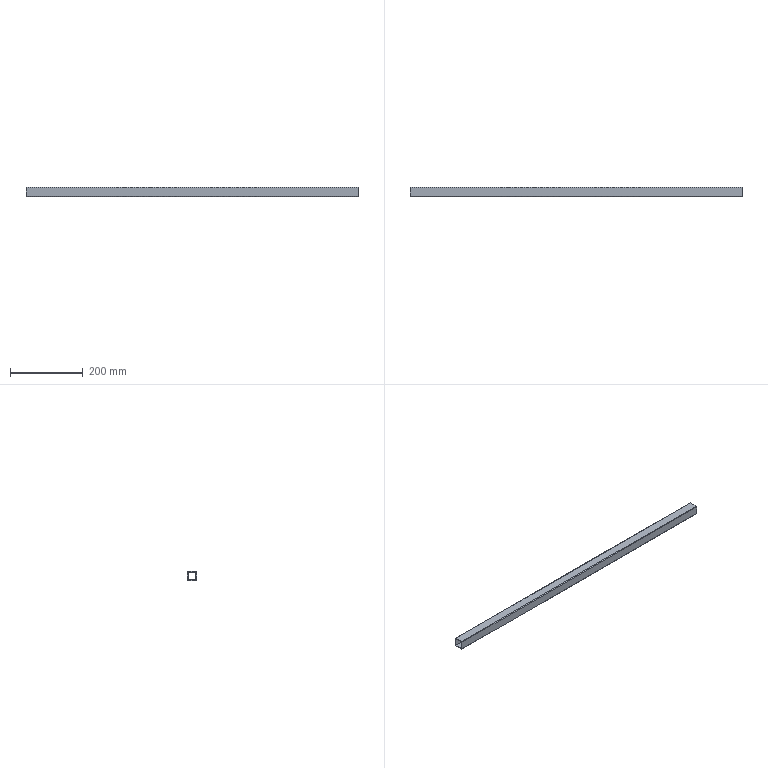Part | NX | features BREP 1 | 1 solid | 14 faces | box 910.59 x 25.4 x 25.4 mm | volume 159055 mm3 | plane 10 | cylinder 4 | commonest cylinder face diameters 3.175 x4
STEP:
#1=CARTESIAN_POINT('',(-455.295,12.7,-11.113));
#2=VERTEX_POINT('',#1);
#3=CARTESIAN_POINT('',(-455.295,12.7,11.113));
#4=VERTEX_POINT('',#3);
#5=CARTESIAN_POINT('',(-455.295,12.7,-11.113));
#6=DIRECTION('',(0.,0.,1.));
#7=VECTOR('',#6,1000.);
#8=LINE('',#5,#7);
#9=EDGE_CURVE('',#2,#4,#8,.T.);
#10=ORIENTED_EDGE('',*,*,#9,.F.);
#11=CARTESIAN_POINT('',(-455.295,11.113,-12.7));
#12=VERTEX_POINT('',#11);
#13=CARTESIAN_POINT('',(-455.295,11.113,-11.113));
#14=DIRECTION('',(-1.,0.,0.));
#15=DIRECTION('',(0.,1.,0.));
#16=AXIS2_PLACEMENT_3D('',#13,#14,#15);
#17=CIRCLE('',#16,1.587);
#18=EDGE_CURVE('',#2,#12,#17,.T.);
#19=ORIENTED_EDGE('',*,*,#18,.T.);
#20=CARTESIAN_POINT('',(-455.295,-11.113,-12.7));
#21=VERTEX_POINT('',#20);
#22=CARTESIAN_POINT('',(-455.295,-11.113,-12.7));
#23=DIRECTION('',(0.,1.,0.));
#24=VECTOR('',#23,1000.);
#25=LINE('',#22,#24);
#26=EDGE_CURVE('',#21,#12,#25,.T.);
#27=ORIENTED_EDGE('',*,*,#26,.F.);
#28=CARTESIAN_POINT('',(-455.295,-12.7,-11.113));
#29=VERTEX_POINT('',#28);
#30=CARTESIAN_POINT('',(-455.295,-11.113,-11.113));
#31=DIRECTION('',(-1.,0.,0.));
#32=DIRECTION('',(0.,0.,-1.));
#33=AXIS2_PLACEMENT_3D('',#30,#31,#32);
#34=CIRCLE('',#33,1.587);
#35=EDGE_CURVE('',#21,#29,#34,.T.);
#36=ORIENTED_EDGE('',*,*,#35,.T.);
#37=CARTESIAN_POINT('',(-455.295,-12.7,11.113));
#38=VERTEX_POINT('',#37);
#39=CARTESIAN_POINT('',(-455.295,-12.7,11.113));
#40=DIRECTION('',(0.,0.,-1.));
#41=VECTOR('',#40,1000.);
#42=LINE('',#39,#41);
#43=EDGE_CURVE('',#38,#29,#42,.T.);
#44=ORIENTED_EDGE('',*,*,#43,.F.);
#45=CARTESIAN_POINT('',(-455.295,-11.113,12.7));
#46=VERTEX_POINT('',#45);
#47=CARTESIAN_POINT('',(-455.295,-11.113,11.113));
#48=DIRECTION('',(-1.,0.,0.));
#49=DIRECTION('',(0.,-1.,0.));
#50=AXIS2_PLACEMENT_3D('',#47,#48,#49);
#51=CIRCLE('',#50,1.587);
#52=EDGE_CURVE('',#38,#46,#51,.T.);
#53=ORIENTED_EDGE('',*,*,#52,.T.);
#54=CARTESIAN_POINT('',(-455.295,11.113,12.7));
#55=VERTEX_POINT('',#54);
#56=CARTESIAN_POINT('',(-455.295,11.113,12.7));
#57=DIRECTION('',(0.,-1.,0.));
#58=VECTOR('',#57,1000.);
#59=LINE('',#56,#58);
#60=EDGE_CURVE('',#55,#46,#59,.T.);
#61=ORIENTED_EDGE('',*,*,#60,.F.);
#62=CARTESIAN_POINT('',(-455.295,11.113,11.113));
#63=DIRECTION('',(-1.,0.,0.));
#64=DIRECTION('',(0.,0.,1.));
#65=AXIS2_PLACEMENT_3D('',#62,#63,#64);
#66=CIRCLE('',#65,1.587);
#67=EDGE_CURVE('',#55,#4,#66,.T.);
#68=ORIENTED_EDGE('',*,*,#67,.T.);
#69=EDGE_LOOP('',(#10,#19,#27,#36,#44,#53,#61,#68));
#70=FACE_BOUND('',#69,.T.);
#71=CARTESIAN_POINT('',(-455.295,10.82,10.82));
#72=VERTEX_POINT('',#71);
#73=CARTESIAN_POINT('',(-455.295,10.82,-10.82));
#74=VERTEX_POINT('',#73);
#75=CARTESIAN_POINT('',(-455.295,10.82,10.82));
#76=DIRECTION('',(0.,0.,-1.));
#77=VECTOR('',#76,1000.);
#78=LINE('',#75,#77);
#79=EDGE_CURVE('',#72,#74,#78,.T.);
#80=ORIENTED_EDGE('',*,*,#79,.F.);
#81=CARTESIAN_POINT('',(-455.295,-10.82,10.82));
#82=VERTEX_POINT('',#81);
#83=CARTESIAN_POINT('',(-455.295,-10.82,10.82));
#84=DIRECTION('',(0.,1.,0.));
#85=VECTOR('',#84,1000.);
#86=LINE('',#83,#85);
#87=EDGE_CURVE('',#82,#72,#86,.T.);
#88=ORIENTED_EDGE('',*,*,#87,.F.);
#89=CARTESIAN_POINT('',(-455.295,-10.82,-10.82));
#90=VERTEX_POINT('',#89);
#91=CARTESIAN_POINT('',(-455.295,-10.82,-10.82));
#92=DIRECTION('',(0.,0.,1.));
#93=VECTOR('',#92,1000.);
#94=LINE('',#91,#93);
#95=EDGE_CURVE('',#90,#82,#94,.T.);
#96=ORIENTED_EDGE('',*,*,#95,.F.);
#97=CARTESIAN_POINT('',(-455.295,10.82,-10.82));
#98=DIRECTION('',(0.,-1.,0.));
#99=VECTOR('',#98,1000.);
#100=LINE('',#97,#99);
#101=EDGE_CURVE('',#74,#90,#100,.T.);
#102=ORIENTED_EDGE('',*,*,#101,.F.);
#103=EDGE_LOOP('',(#80,#88,#96,#102));
#104=FACE_BOUND('',#103,.T.);
#105=CARTESIAN_POINT('',(-455.295,0.,0.));
#106=DIRECTION('',(1.,0.,0.));
#107=DIRECTION('',(0.,1.,0.));
#108=AXIS2_PLACEMENT_3D('',#105,#106,#107);
#109=PLANE('',#108);
#110=ADVANCED_FACE('',(#70,#104),#109,.F.);
#111=CARTESIAN_POINT('',(455.295,-10.82,-10.82));
#112=VERTEX_POINT('',#111);
#113=CARTESIAN_POINT('',(-455.295,-10.82,-10.82));
#114=DIRECTION('',(1.,0.,0.));
#115=VECTOR('',#114,1000.);
#116=LINE('',#113,#115);
#117=EDGE_CURVE('',#90,#112,#116,.T.);
#118=ORIENTED_EDGE('',*,*,#117,.T.);
#119=CARTESIAN_POINT('',(455.295,10.82,-10.82));
#120=VERTEX_POINT('',#119);
#121=CARTESIAN_POINT('',(455.295,10.82,-10.82));
#122=DIRECTION('',(0.,-1.,0.));
#123=VECTOR('',#122,1000.);
#124=LINE('',#121,#123);
#125=EDGE_CURVE('',#120,#112,#124,.T.);
#126=ORIENTED_EDGE('',*,*,#125,.F.);
#127=CARTESIAN_POINT('',(-455.295,10.82,-10.82));
#128=DIRECTION('',(1.,0.,0.));
#129=VECTOR('',#128,1000.);
#130=LINE('',#127,#129);
#131=EDGE_CURVE('',#74,#120,#130,.T.);
#132=ORIENTED_EDGE('',*,*,#131,.F.);
#133=ORIENTED_EDGE('',*,*,#101,.T.);
#134=EDGE_LOOP('',(#118,#126,#132,#133));
#135=FACE_BOUND('',#134,.T.);
#136=CARTESIAN_POINT('',(-455.295,10.82,-10.82));
#137=DIRECTION('',(0.,0.,1.));
#138=DIRECTION('',(1.,0.,0.));
#139=AXIS2_PLACEMENT_3D('',#136,#137,#138);
#140=PLANE('',#139);
#141=ADVANCED_FACE('',(#135),#140,.T.);
#142=ORIENTED_EDGE('',*,*,#131,.T.);
#143=CARTESIAN_POINT('',(455.295,10.82,10.82));
#144=VERTEX_POINT('',#143);
#145=CARTESIAN_POINT('',(455.295,10.82,10.82));
#146=DIRECTION('',(0.,0.,-1.));
#147=VECTOR('',#146,1000.);
#148=LINE('',#145,#147);
#149=EDGE_CURVE('',#144,#120,#148,.T.);
#150=ORIENTED_EDGE('',*,*,#149,.F.);
#151=CARTESIAN_POINT('',(-455.295,10.82,10.82));
#152=DIRECTION('',(1.,0.,0.));
#153=VECTOR('',#152,1000.);
#154=LINE('',#151,#153);
#155=EDGE_CURVE('',#72,#144,#154,.T.);
#156=ORIENTED_EDGE('',*,*,#155,.F.);
#157=ORIENTED_EDGE('',*,*,#79,.T.);
#158=EDGE_LOOP('',(#142,#150,#156,#157));
#159=FACE_BOUND('',#158,.T.);
#160=CARTESIAN_POINT('',(-455.295,10.82,10.82));
#161=DIRECTION('',(0.,-1.,0.));
#162=DIRECTION('',(0.,0.,-1.));
#163=AXIS2_PLACEMENT_3D('',#160,#161,#162);
#164=PLANE('',#163);
#165=ADVANCED_FACE('',(#159),#164,.T.);
#166=ORIENTED_EDGE('',*,*,#155,.T.);
#167=CARTESIAN_POINT('',(455.295,-10.82,10.82));
#168=VERTEX_POINT('',#167);
#169=CARTESIAN_POINT('',(455.295,-10.82,10.82));
#170=DIRECTION('',(0.,1.,0.));
#171=VECTOR('',#170,1000.);
#172=LINE('',#169,#171);
#173=EDGE_CURVE('',#168,#144,#172,.T.);
#174=ORIENTED_EDGE('',*,*,#173,.F.);
#175=CARTESIAN_POINT('',(-455.295,-10.82,10.82));
#176=DIRECTION('',(1.,0.,0.));
#177=VECTOR('',#176,1000.);
#178=LINE('',#175,#177);
#179=EDGE_CURVE('',#82,#168,#178,.T.);
#180=ORIENTED_EDGE('',*,*,#179,.F.);
#181=ORIENTED_EDGE('',*,*,#87,.T.);
#182=EDGE_LOOP('',(#166,#174,#180,#181));
#183=FACE_BOUND('',#182,.T.);
#184=CARTESIAN_POINT('',(-455.295,-10.82,10.82));
#185=DIRECTION('',(0.,0.,-1.));
#186=DIRECTION('',(0.,-1.,0.));
#187=AXIS2_PLACEMENT_3D('',#184,#185,#186);
#188=PLANE('',#187);
#189=ADVANCED_FACE('',(#183),#188,.T.);
#190=ORIENTED_EDGE('',*,*,#179,.T.);
#191=CARTESIAN_POINT('',(455.295,-10.82,-10.82));
#192=DIRECTION('',(0.,0.,1.));
#193=VECTOR('',#192,1000.);
#194=LINE('',#191,#193);
#195=EDGE_CURVE('',#112,#168,#194,.T.);
#196=ORIENTED_EDGE('',*,*,#195,.F.);
#197=ORIENTED_EDGE('',*,*,#117,.F.);
#198=ORIENTED_EDGE('',*,*,#95,.T.);
#199=EDGE_LOOP('',(#190,#196,#197,#198));
#200=FACE_BOUND('',#199,.T.);
#201=CARTESIAN_POINT('',(-455.295,-10.82,-10.82));
#202=DIRECTION('',(0.,1.,0.));
#203=DIRECTION('',(1.,0.,0.));
#204=AXIS2_PLACEMENT_3D('',#201,#202,#203);
#205=PLANE('',#204);
#206=ADVANCED_FACE('',(#200),#205,.T.);
#207=CARTESIAN_POINT('',(455.295,11.113,12.7));
#208=VERTEX_POINT('',#207);
#209=CARTESIAN_POINT('',(455.295,-11.113,12.7));
#210=VERTEX_POINT('',#209);
#211=CARTESIAN_POINT('',(455.295,11.113,12.7));
#212=DIRECTION('',(0.,-1.,0.));
#213=VECTOR('',#212,1000.);
#214=LINE('',#211,#213);
#215=EDGE_CURVE('',#208,#210,#214,.T.);
#216=ORIENTED_EDGE('',*,*,#215,.T.);
#217=CARTESIAN_POINT('',(455.295,-12.7,11.113));
#218=VERTEX_POINT('',#217);
#219=CARTESIAN_POINT('',(455.295,-11.113,11.113));
#220=DIRECTION('',(1.,0.,0.));
#221=DIRECTION('',(0.,0.,1.));
#222=AXIS2_PLACEMENT_3D('',#219,#220,#221);
#223=CIRCLE('',#222,1.587);
#224=EDGE_CURVE('',#210,#218,#223,.T.);
#225=ORIENTED_EDGE('',*,*,#224,.T.);
#226=CARTESIAN_POINT('',(455.295,-12.7,-11.113));
#227=VERTEX_POINT('',#226);
#228=CARTESIAN_POINT('',(455.295,-12.7,11.113));
#229=DIRECTION('',(0.,0.,-1.));
#230=VECTOR('',#229,1000.);
#231=LINE('',#228,#230);
#232=EDGE_CURVE('',#218,#227,#231,.T.);
#233=ORIENTED_EDGE('',*,*,#232,.T.);
#234=CARTESIAN_POINT('',(455.295,-11.113,-12.7));
#235=VERTEX_POINT('',#234);
#236=CARTESIAN_POINT('',(455.295,-11.113,-11.113));
#237=DIRECTION('',(1.,0.,0.));
#238=DIRECTION('',(0.,-1.,0.));
#239=AXIS2_PLACEMENT_3D('',#236,#237,#238);
#240=CIRCLE('',#239,1.587);
#241=EDGE_CURVE('',#227,#235,#240,.T.);
#242=ORIENTED_EDGE('',*,*,#241,.T.);
#243=CARTESIAN_POINT('',(455.295,11.113,-12.7));
#244=VERTEX_POINT('',#243);
#245=CARTESIAN_POINT('',(455.295,-11.113,-12.7));
#246=DIRECTION('',(0.,1.,0.));
#247=VECTOR('',#246,1000.);
#248=LINE('',#245,#247);
#249=EDGE_CURVE('',#235,#244,#248,.T.);
#250=ORIENTED_EDGE('',*,*,#249,.T.);
#251=CARTESIAN_POINT('',(455.295,12.7,-11.113));
#252=VERTEX_POINT('',#251);
#253=CARTESIAN_POINT('',(455.295,11.113,-11.113));
#254=DIRECTION('',(1.,0.,0.));
#255=DIRECTION('',(0.,0.,-1.));
#256=AXIS2_PLACEMENT_3D('',#253,#254,#255);
#257=CIRCLE('',#256,1.587);
#258=EDGE_CURVE('',#244,#252,#257,.T.);
#259=ORIENTED_EDGE('',*,*,#258,.T.);
#260=CARTESIAN_POINT('',(455.295,12.7,11.113));
#261=VERTEX_POINT('',#260);
#262=CARTESIAN_POINT('',(455.295,12.7,-11.113));
#263=DIRECTION('',(0.,0.,1.));
#264=VECTOR('',#263,1000.);
#265=LINE('',#262,#264);
#266=EDGE_CURVE('',#252,#261,#265,.T.);
#267=ORIENTED_EDGE('',*,*,#266,.T.);
#268=CARTESIAN_POINT('',(455.295,11.113,11.113));
#269=DIRECTION('',(1.,0.,0.));
#270=DIRECTION('',(0.,1.,0.));
#271=AXIS2_PLACEMENT_3D('',#268,#269,#270);
#272=CIRCLE('',#271,1.587);
#273=EDGE_CURVE('',#261,#208,#272,.T.);
#274=ORIENTED_EDGE('',*,*,#273,.T.);
#275=EDGE_LOOP('',(#216,#225,#233,#242,#250,#259,#267,#274));
#276=FACE_BOUND('',#275,.T.);
#277=ORIENTED_EDGE('',*,*,#195,.T.);
#278=ORIENTED_EDGE('',*,*,#173,.T.);
#279=ORIENTED_EDGE('',*,*,#149,.T.);
#280=ORIENTED_EDGE('',*,*,#125,.T.);
#281=EDGE_LOOP('',(#277,#278,#279,#280));
#282=FACE_BOUND('',#281,.T.);
#283=CARTESIAN_POINT('',(455.295,0.,0.));
#284=DIRECTION('',(1.,0.,0.));
#285=DIRECTION('',(0.,1.,0.));
#286=AXIS2_PLACEMENT_3D('',#283,#284,#285);
#287=PLANE('',#286);
#288=ADVANCED_FACE('',(#276,#282),#287,.T.);
#289=ORIENTED_EDGE('',*,*,#273,.F.);
#290=CARTESIAN_POINT('',(455.295,12.7,11.113));
#291=DIRECTION('',(-1.,0.,0.));
#292=VECTOR('',#291,1000.);
#293=LINE('',#290,#292);
#294=EDGE_CURVE('',#261,#4,#293,.T.);
#295=ORIENTED_EDGE('',*,*,#294,.T.);
#296=ORIENTED_EDGE('',*,*,#67,.F.);
#297=CARTESIAN_POINT('',(455.295,11.113,12.7));
#298=DIRECTION('',(-1.,0.,0.));
#299=VECTOR('',#298,1000.);
#300=LINE('',#297,#299);
#301=EDGE_CURVE('',#208,#55,#300,.T.);
#302=ORIENTED_EDGE('',*,*,#301,.F.);
#303=EDGE_LOOP('',(#289,#295,#296,#302));
#304=FACE_BOUND('',#303,.T.);
#305=CARTESIAN_POINT('',(456.721,11.113,11.113));
#306=DIRECTION('',(-1.,0.,0.));
#307=DIRECTION('',(0.,0.,1.));
#308=AXIS2_PLACEMENT_3D('',#305,#306,#307);
#309=CYLINDRICAL_SURFACE('',#308,1.587);
#310=ADVANCED_FACE('',(#304),#309,.T.);
#311=ORIENTED_EDGE('',*,*,#60,.T.);
#312=CARTESIAN_POINT('',(455.295,-11.113,12.7));
#313=DIRECTION('',(-1.,0.,0.));
#314=VECTOR('',#313,1000.);
#315=LINE('',#312,#314);
#316=EDGE_CURVE('',#210,#46,#315,.T.);
#317=ORIENTED_EDGE('',*,*,#316,.F.);
#318=ORIENTED_EDGE('',*,*,#215,.F.);
#319=ORIENTED_EDGE('',*,*,#301,.T.);
#320=EDGE_LOOP('',(#311,#317,#318,#319));
#321=FACE_BOUND('',#320,.T.);
#322=CARTESIAN_POINT('',(-455.295,12.7,12.7));
#323=DIRECTION('',(0.,0.,1.));
#324=DIRECTION('',(1.,0.,0.));
#325=AXIS2_PLACEMENT_3D('',#322,#323,#324);
#326=PLANE('',#325);
#327=ADVANCED_FACE('',(#321),#326,.T.);
#328=ORIENTED_EDGE('',*,*,#224,.F.);
#329=ORIENTED_EDGE('',*,*,#316,.T.);
#330=ORIENTED_EDGE('',*,*,#52,.F.);
#331=CARTESIAN_POINT('',(455.295,-12.7,11.113));
#332=DIRECTION('',(-1.,0.,0.));
#333=VECTOR('',#332,1000.);
#334=LINE('',#331,#333);
#335=EDGE_CURVE('',#218,#38,#334,.T.);
#336=ORIENTED_EDGE('',*,*,#335,.F.);
#337=EDGE_LOOP('',(#328,#329,#330,#336));
#338=FACE_BOUND('',#337,.T.);
#339=CARTESIAN_POINT('',(456.721,-11.113,11.113));
#340=DIRECTION('',(-1.,0.,0.));
#341=DIRECTION('',(0.,-1.,0.));
#342=AXIS2_PLACEMENT_3D('',#339,#340,#341);
#343=CYLINDRICAL_SURFACE('',#342,1.587);
#344=ADVANCED_FACE('',(#338),#343,.T.);
#345=ORIENTED_EDGE('',*,*,#43,.T.);
#346=CARTESIAN_POINT('',(455.295,-12.7,-11.113));
#347=DIRECTION('',(-1.,0.,0.));
#348=VECTOR('',#347,1000.);
#349=LINE('',#346,#348);
#350=EDGE_CURVE('',#227,#29,#349,.T.);
#351=ORIENTED_EDGE('',*,*,#350,.F.);
#352=ORIENTED_EDGE('',*,*,#232,.F.);
#353=ORIENTED_EDGE('',*,*,#335,.T.);
#354=EDGE_LOOP('',(#345,#351,#352,#353));
#355=FACE_BOUND('',#354,.T.);
#356=CARTESIAN_POINT('',(-455.295,-12.7,12.7));
#357=DIRECTION('',(0.,-1.,0.));
#358=DIRECTION('',(0.,0.,-1.));
#359=AXIS2_PLACEMENT_3D('',#356,#357,#358);
#360=PLANE('',#359);
#361=ADVANCED_FACE('',(#355),#360,.T.);
#362=ORIENTED_EDGE('',*,*,#241,.F.);
#363=ORIENTED_EDGE('',*,*,#350,.T.);
#364=ORIENTED_EDGE('',*,*,#35,.F.);
#365=CARTESIAN_POINT('',(455.295,-11.113,-12.7));
#366=DIRECTION('',(-1.,0.,0.));
#367=VECTOR('',#366,1000.);
#368=LINE('',#365,#367);
#369=EDGE_CURVE('',#235,#21,#368,.T.);
#370=ORIENTED_EDGE('',*,*,#369,.F.);
#371=EDGE_LOOP('',(#362,#363,#364,#370));
#372=FACE_BOUND('',#371,.T.);
#373=CARTESIAN_POINT('',(456.721,-11.113,-11.113));
#374=DIRECTION('',(-1.,0.,0.));
#375=DIRECTION('',(0.,0.,-1.));
#376=AXIS2_PLACEMENT_3D('',#373,#374,#375);
#377=CYLINDRICAL_SURFACE('',#376,1.587);
#378=ADVANCED_FACE('',(#372),#377,.T.);
#379=ORIENTED_EDGE('',*,*,#249,.F.);
#380=ORIENTED_EDGE('',*,*,#369,.T.);
#381=ORIENTED_EDGE('',*,*,#26,.T.);
#382=CARTESIAN_POINT('',(455.295,11.113,-12.7));
#383=DIRECTION('',(-1.,0.,0.));
#384=VECTOR('',#383,1000.);
#385=LINE('',#382,#384);
#386=EDGE_CURVE('',#244,#12,#385,.T.);
#387=ORIENTED_EDGE('',*,*,#386,.F.);
#388=EDGE_LOOP('',(#379,#380,#381,#387));
#389=FACE_BOUND('',#388,.T.);
#390=CARTESIAN_POINT('',(-455.295,-12.7,-12.7));
#391=DIRECTION('',(0.,0.,-1.));
#392=DIRECTION('',(0.,-1.,0.));
#393=AXIS2_PLACEMENT_3D('',#390,#391,#392);
#394=PLANE('',#393);
#395=ADVANCED_FACE('',(#389),#394,.T.);
#396=ORIENTED_EDGE('',*,*,#258,.F.);
#397=ORIENTED_EDGE('',*,*,#386,.T.);
#398=ORIENTED_EDGE('',*,*,#18,.F.);
#399=CARTESIAN_POINT('',(455.295,12.7,-11.113));
#400=DIRECTION('',(-1.,0.,0.));
#401=VECTOR('',#400,1000.);
#402=LINE('',#399,#401);
#403=EDGE_CURVE('',#252,#2,#402,.T.);
#404=ORIENTED_EDGE('',*,*,#403,.F.);
#405=EDGE_LOOP('',(#396,#397,#398,#404));
#406=FACE_BOUND('',#405,.T.);
#407=CARTESIAN_POINT('',(456.721,11.113,-11.113));
#408=DIRECTION('',(-1.,0.,0.));
#409=DIRECTION('',(0.,1.,0.));
#410=AXIS2_PLACEMENT_3D('',#407,#408,#409);
#411=CYLINDRICAL_SURFACE('',#410,1.587);
#412=ADVANCED_FACE('',(#406),#411,.T.);
#413=ORIENTED_EDGE('',*,*,#266,.F.);
#414=ORIENTED_EDGE('',*,*,#403,.T.);
#415=ORIENTED_EDGE('',*,*,#9,.T.);
#416=ORIENTED_EDGE('',*,*,#294,.F.);
#417=EDGE_LOOP('',(#413,#414,#415,#416));
#418=FACE_BOUND('',#417,.T.);
#419=CARTESIAN_POINT('',(-455.295,12.7,-12.7));
#420=DIRECTION('',(0.,1.,0.));
#421=DIRECTION('',(1.,0.,0.));
#422=AXIS2_PLACEMENT_3D('',#419,#420,#421);
#423=PLANE('',#422);
#424=ADVANCED_FACE('',(#418),#423,.T.);
#425=CLOSED_SHELL('',(#110,#141,#165,#189,#206,#288,#310,#327,#344,#361,#378,#395,#412,#424));
#426=MANIFOLD_SOLID_BREP('',#425);
#427=(LENGTH_UNIT()NAMED_UNIT(*)SI_UNIT(.MILLI.,.METRE.));
#428=UNCERTAINTY_MEASURE_WITH_UNIT(LENGTH_MEASURE(0.00001),#427,'','');
#429=(NAMED_UNIT(*)PLANE_ANGLE_UNIT()SI_UNIT($,.RADIAN.));
#430=(NAMED_UNIT(*)SI_UNIT($,.STERADIAN.)SOLID_ANGLE_UNIT());
#431=(GEOMETRIC_REPRESENTATION_CONTEXT(3)GLOBAL_UNCERTAINTY_ASSIGNED_CONTEXT((#428))GLOBAL_UNIT_ASSIGNED_CONTEXT((#427,#429,#430))REPRESENTATION_CONTEXT('',''));
#432=ADVANCED_BREP_SHAPE_REPRESENTATION('',(#426),#431);